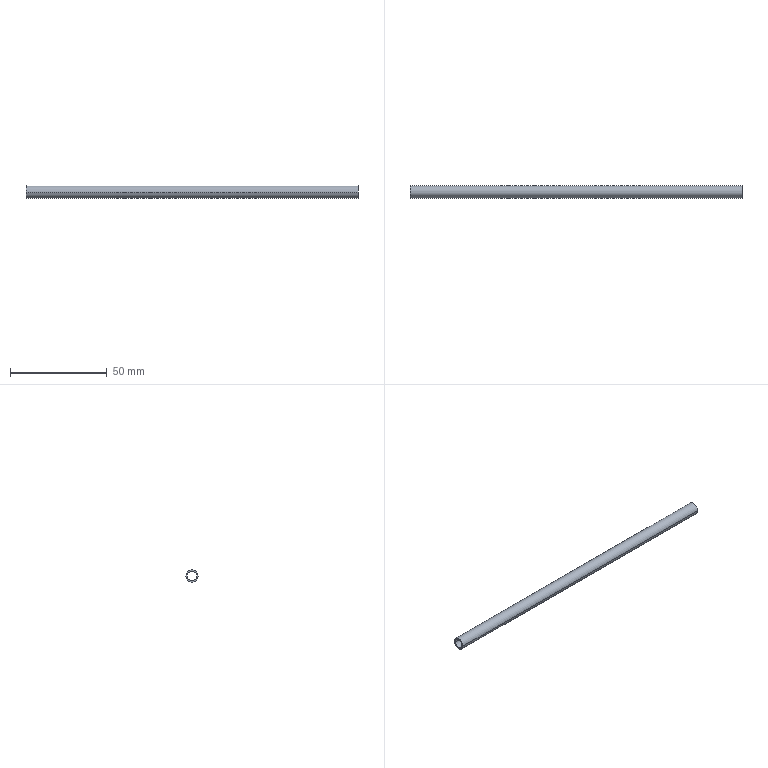Part | STEP file | copper tube 31_default_machined_ | 1 solid | 6 faces | box 172 x 6.35 x 6.35 mm | volume 2399 mm3 | cylinder 4 | plane 2 | commonest cylinder face diameters 4.75 x2 6.35 x2
STEP:
#1=CARTESIAN_POINT('',(0.,0.,0.));
#2=DIRECTION('',(0.,0.,1.));
#3=DIRECTION('',(1.,0.,0.));
#4=AXIS2_PLACEMENT_3D('',#1,#2,#3);
#5=CARTESIAN_POINT('',(-142.,3.175,0.));
#6=VERTEX_POINT('',#5);
#7=CARTESIAN_POINT('',(-142.,-3.175,0.));
#8=VERTEX_POINT('',#7);
#9=CARTESIAN_POINT('',(-142.,0.,0.));
#10=DIRECTION('',(1.,0.,0.));
#11=DIRECTION('',(0.,1.,0.));
#12=AXIS2_PLACEMENT_3D('',#9,#10,#11);
#13=CIRCLE('',#12,3.175);
#14=CARTESIAN_POINT('',(-142.,0.,0.));
#15=DIRECTION('',(1.,0.,0.));
#16=DIRECTION('',(0.,1.,0.));
#17=AXIS2_PLACEMENT_3D('',#14,#15,#16);
#18=CYLINDRICAL_SURFACE('',#17,3.175);
#19=CARTESIAN_POINT('',(0.,0.));
#20=DIRECTION('',(1.,0.));
#21=VECTOR('',#20,1.);
#22=LINE('',#19,#21);
#23=(GEOMETRIC_REPRESENTATION_CONTEXT(2)PARAMETRIC_REPRESENTATION_CONTEXT()REPRESENTATION_CONTEXT('',''));
#24=DEFINITIONAL_REPRESENTATION('',(#22),#23);
#25=PCURVE('',#18,#24);
#26=CARTESIAN_POINT('',(-142.,0.,0.));
#27=DIRECTION('',(-1.,0.,0.));
#28=DIRECTION('',(0.,-1.,0.));
#29=AXIS2_PLACEMENT_3D('',#26,#27,#28);
#30=PLANE('',#29);
#31=CARTESIAN_POINT('',(-3.175,0.));
#32=CARTESIAN_POINT('',(-3.175,5.499));
#33=CARTESIAN_POINT('',(1.587,2.75));
#34=CARTESIAN_POINT('',(6.35,0.));
#35=CARTESIAN_POINT('',(1.587,-2.75));
#36=CARTESIAN_POINT('',(-3.175,-5.499));
#37=CARTESIAN_POINT('',(-3.175,0.));
#38=(BOUNDED_CURVE()B_SPLINE_CURVE(2,(#31,#32,#33,#34,#35,#36,#37),.UNSPECIFIED.,.T.,.F.)B_SPLINE_CURVE_WITH_KNOTS((1,2,2,2,2,1),(-2.094,0.,2.094,4.189,6.283,8.378),.UNSPECIFIED.)CURVE()GEOMETRIC_REPRESENTATION_ITEM()RATIONAL_B_SPLINE_CURVE((1.,0.5,1.,0.5,1.,0.5,1.))REPRESENTATION_ITEM(''));
#39=(GEOMETRIC_REPRESENTATION_CONTEXT(2)PARAMETRIC_REPRESENTATION_CONTEXT()REPRESENTATION_CONTEXT('',''));
#40=DEFINITIONAL_REPRESENTATION('',(#38),#39);
#41=PCURVE('',#30,#40);
#42=SURFACE_CURVE('',#13,(#25,#41),.PCURVE_S1.);
#43=EDGE_CURVE('',#6,#8,#42,.T.);
#44=ORIENTED_EDGE('',*,*,#43,.T.);
#45=CARTESIAN_POINT('',(30.,-3.175,0.));
#46=VERTEX_POINT('',#45);
#47=CARTESIAN_POINT('',(-142.,-3.175,0.));
#48=DIRECTION('',(1.,0.,0.));
#49=VECTOR('',#48,1.);
#50=LINE('',#47,#49);
#51=CARTESIAN_POINT('',(3.142,0.));
#52=DIRECTION('',(0.,1.));
#53=VECTOR('',#52,1.);
#54=LINE('',#51,#53);
#55=(GEOMETRIC_REPRESENTATION_CONTEXT(2)PARAMETRIC_REPRESENTATION_CONTEXT()REPRESENTATION_CONTEXT('',''));
#56=DEFINITIONAL_REPRESENTATION('',(#54),#55);
#57=PCURVE('',#18,#56);
#58=CARTESIAN_POINT('',(-142.,0.,0.));
#59=DIRECTION('',(1.,0.,0.));
#60=DIRECTION('',(0.,1.,0.));
#61=AXIS2_PLACEMENT_3D('',#58,#59,#60);
#62=CYLINDRICAL_SURFACE('',#61,3.175);
#63=CARTESIAN_POINT('',(3.142,0.));
#64=DIRECTION('',(0.,1.));
#65=VECTOR('',#64,1.);
#66=LINE('',#63,#65);
#67=(GEOMETRIC_REPRESENTATION_CONTEXT(2)PARAMETRIC_REPRESENTATION_CONTEXT()REPRESENTATION_CONTEXT('',''));
#68=DEFINITIONAL_REPRESENTATION('',(#66),#67);
#69=PCURVE('',#62,#68);
#70=SURFACE_CURVE('',#50,(#57,#69),.PCURVE_S1.);
#71=EDGE_CURVE('',#8,#46,#70,.T.);
#72=ORIENTED_EDGE('',*,*,#71,.T.);
#73=CARTESIAN_POINT('',(30.,3.175,0.));
#74=VERTEX_POINT('',#73);
#75=CARTESIAN_POINT('',(30.,0.,0.));
#76=DIRECTION('',(1.,0.,0.));
#77=DIRECTION('',(0.,1.,0.));
#78=AXIS2_PLACEMENT_3D('',#75,#76,#77);
#79=CIRCLE('',#78,3.175);
#80=CARTESIAN_POINT('',(0.,172.));
#81=DIRECTION('',(1.,0.));
#82=VECTOR('',#81,1.);
#83=LINE('',#80,#82);
#84=(GEOMETRIC_REPRESENTATION_CONTEXT(2)PARAMETRIC_REPRESENTATION_CONTEXT()REPRESENTATION_CONTEXT('',''));
#85=DEFINITIONAL_REPRESENTATION('',(#83),#84);
#86=PCURVE('',#18,#85);
#87=CARTESIAN_POINT('',(30.,0.,0.));
#88=DIRECTION('',(1.,0.,0.));
#89=DIRECTION('',(0.,1.,0.));
#90=AXIS2_PLACEMENT_3D('',#87,#88,#89);
#91=PLANE('',#90);
#92=CARTESIAN_POINT('',(0.,0.));
#93=DIRECTION('',(1.,0.));
#94=AXIS2_PLACEMENT_2D('',#92,#93);
#95=CIRCLE('',#94,3.175);
#96=(GEOMETRIC_REPRESENTATION_CONTEXT(2)PARAMETRIC_REPRESENTATION_CONTEXT()REPRESENTATION_CONTEXT('',''));
#97=DEFINITIONAL_REPRESENTATION('',(#95),#96);
#98=PCURVE('',#91,#97);
#99=SURFACE_CURVE('',#79,(#86,#98),.PCURVE_S1.);
#100=EDGE_CURVE('',#74,#46,#99,.T.);
#101=ORIENTED_EDGE('',*,*,#100,.F.);
#102=CARTESIAN_POINT('',(-142.,3.175,0.));
#103=DIRECTION('',(1.,0.,0.));
#104=VECTOR('',#103,1.);
#105=LINE('',#102,#104);
#106=CARTESIAN_POINT('',(0.,0.));
#107=DIRECTION('',(0.,1.));
#108=VECTOR('',#107,1.);
#109=LINE('',#106,#108);
#110=(GEOMETRIC_REPRESENTATION_CONTEXT(2)PARAMETRIC_REPRESENTATION_CONTEXT()REPRESENTATION_CONTEXT('',''));
#111=DEFINITIONAL_REPRESENTATION('',(#109),#110);
#112=PCURVE('',#18,#111);
#113=CARTESIAN_POINT('',(6.283,0.));
#114=DIRECTION('',(0.,1.));
#115=VECTOR('',#114,1.);
#116=LINE('',#113,#115);
#117=(GEOMETRIC_REPRESENTATION_CONTEXT(2)PARAMETRIC_REPRESENTATION_CONTEXT()REPRESENTATION_CONTEXT('',''));
#118=DEFINITIONAL_REPRESENTATION('',(#116),#117);
#119=PCURVE('',#62,#118);
#120=SURFACE_CURVE('',#105,(#112,#119),.PCURVE_S1.);
#121=EDGE_CURVE('',#6,#74,#120,.T.);
#122=ORIENTED_EDGE('',*,*,#121,.F.);
#123=EDGE_LOOP('',(#44,#72,#101,#122));
#124=FACE_BOUND('',#123,.T.);
#125=ADVANCED_FACE('',(#124),#18,.T.);
#126=CARTESIAN_POINT('',(-142.,2.375,0.));
#127=VERTEX_POINT('',#126);
#128=CARTESIAN_POINT('',(30.,2.375,0.));
#129=VERTEX_POINT('',#128);
#130=CARTESIAN_POINT('',(-142.,2.375,0.));
#131=DIRECTION('',(1.,0.,0.));
#132=VECTOR('',#131,1.);
#133=LINE('',#130,#132);
#134=CARTESIAN_POINT('',(-142.,0.,0.));
#135=DIRECTION('',(1.,0.,0.));
#136=DIRECTION('',(0.,1.,0.));
#137=AXIS2_PLACEMENT_3D('',#134,#135,#136);
#138=CYLINDRICAL_SURFACE('',#137,2.375);
#139=CARTESIAN_POINT('',(6.283,0.));
#140=DIRECTION('',(0.,1.));
#141=VECTOR('',#140,1.);
#142=LINE('',#139,#141);
#143=(GEOMETRIC_REPRESENTATION_CONTEXT(2)PARAMETRIC_REPRESENTATION_CONTEXT()REPRESENTATION_CONTEXT('',''));
#144=DEFINITIONAL_REPRESENTATION('',(#142),#143);
#145=PCURVE('',#138,#144);
#146=CARTESIAN_POINT('',(-142.,0.,0.));
#147=DIRECTION('',(1.,0.,0.));
#148=DIRECTION('',(0.,1.,0.));
#149=AXIS2_PLACEMENT_3D('',#146,#147,#148);
#150=CYLINDRICAL_SURFACE('',#149,2.375);
#151=CARTESIAN_POINT('',(0.,0.));
#152=DIRECTION('',(0.,1.));
#153=VECTOR('',#152,1.);
#154=LINE('',#151,#153);
#155=(GEOMETRIC_REPRESENTATION_CONTEXT(2)PARAMETRIC_REPRESENTATION_CONTEXT()REPRESENTATION_CONTEXT('',''));
#156=DEFINITIONAL_REPRESENTATION('',(#154),#155);
#157=PCURVE('',#150,#156);
#158=SURFACE_CURVE('',#133,(#145,#157),.PCURVE_S1.);
#159=EDGE_CURVE('',#127,#129,#158,.T.);
#160=ORIENTED_EDGE('',*,*,#159,.T.);
#161=CARTESIAN_POINT('',(30.,-2.375,0.));
#162=VERTEX_POINT('',#161);
#163=CARTESIAN_POINT('',(30.,0.,0.));
#164=DIRECTION('',(1.,0.,0.));
#165=DIRECTION('',(0.,1.,0.));
#166=AXIS2_PLACEMENT_3D('',#163,#164,#165);
#167=CIRCLE('',#166,2.375);
#168=CARTESIAN_POINT('',(0.,172.));
#169=DIRECTION('',(1.,0.));
#170=VECTOR('',#169,1.);
#171=LINE('',#168,#170);
#172=(GEOMETRIC_REPRESENTATION_CONTEXT(2)PARAMETRIC_REPRESENTATION_CONTEXT()REPRESENTATION_CONTEXT('',''));
#173=DEFINITIONAL_REPRESENTATION('',(#171),#172);
#174=PCURVE('',#138,#173);
#175=CARTESIAN_POINT('',(0.,0.));
#176=DIRECTION('',(1.,0.));
#177=AXIS2_PLACEMENT_2D('',#175,#176);
#178=CIRCLE('',#177,2.375);
#179=(GEOMETRIC_REPRESENTATION_CONTEXT(2)PARAMETRIC_REPRESENTATION_CONTEXT()REPRESENTATION_CONTEXT('',''));
#180=DEFINITIONAL_REPRESENTATION('',(#178),#179);
#181=PCURVE('',#91,#180);
#182=SURFACE_CURVE('',#167,(#174,#181),.PCURVE_S1.);
#183=EDGE_CURVE('',#162,#129,#182,.T.);
#184=ORIENTED_EDGE('',*,*,#183,.F.);
#185=CARTESIAN_POINT('',(-142.,-2.375,0.));
#186=VERTEX_POINT('',#185);
#187=CARTESIAN_POINT('',(-142.,-2.375,0.));
#188=DIRECTION('',(1.,0.,0.));
#189=VECTOR('',#188,1.);
#190=LINE('',#187,#189);
#191=CARTESIAN_POINT('',(3.142,0.));
#192=DIRECTION('',(0.,1.));
#193=VECTOR('',#192,1.);
#194=LINE('',#191,#193);
#195=(GEOMETRIC_REPRESENTATION_CONTEXT(2)PARAMETRIC_REPRESENTATION_CONTEXT()REPRESENTATION_CONTEXT('',''));
#196=DEFINITIONAL_REPRESENTATION('',(#194),#195);
#197=PCURVE('',#138,#196);
#198=CARTESIAN_POINT('',(3.142,0.));
#199=DIRECTION('',(0.,1.));
#200=VECTOR('',#199,1.);
#201=LINE('',#198,#200);
#202=(GEOMETRIC_REPRESENTATION_CONTEXT(2)PARAMETRIC_REPRESENTATION_CONTEXT()REPRESENTATION_CONTEXT('',''));
#203=DEFINITIONAL_REPRESENTATION('',(#201),#202);
#204=PCURVE('',#150,#203);
#205=SURFACE_CURVE('',#190,(#197,#204),.PCURVE_S1.);
#206=EDGE_CURVE('',#186,#162,#205,.T.);
#207=ORIENTED_EDGE('',*,*,#206,.F.);
#208=CARTESIAN_POINT('',(-142.,0.,0.));
#209=DIRECTION('',(1.,0.,0.));
#210=DIRECTION('',(0.,1.,0.));
#211=AXIS2_PLACEMENT_3D('',#208,#209,#210);
#212=CIRCLE('',#211,2.375);
#213=CARTESIAN_POINT('',(0.,0.));
#214=DIRECTION('',(1.,0.));
#215=VECTOR('',#214,1.);
#216=LINE('',#213,#215);
#217=(GEOMETRIC_REPRESENTATION_CONTEXT(2)PARAMETRIC_REPRESENTATION_CONTEXT()REPRESENTATION_CONTEXT('',''));
#218=DEFINITIONAL_REPRESENTATION('',(#216),#217);
#219=PCURVE('',#138,#218);
#220=CARTESIAN_POINT('',(-2.375,0.));
#221=CARTESIAN_POINT('',(-2.375,4.114));
#222=CARTESIAN_POINT('',(1.188,2.057));
#223=CARTESIAN_POINT('',(4.75,0.));
#224=CARTESIAN_POINT('',(1.188,-2.057));
#225=CARTESIAN_POINT('',(-2.375,-4.114));
#226=CARTESIAN_POINT('',(-2.375,0.));
#227=(BOUNDED_CURVE()B_SPLINE_CURVE(2,(#220,#221,#222,#223,#224,#225,#226),.UNSPECIFIED.,.T.,.F.)B_SPLINE_CURVE_WITH_KNOTS((1,2,2,2,2,1),(-2.094,0.,2.094,4.189,6.283,8.378),.UNSPECIFIED.)CURVE()GEOMETRIC_REPRESENTATION_ITEM()RATIONAL_B_SPLINE_CURVE((1.,0.5,1.,0.5,1.,0.5,1.))REPRESENTATION_ITEM(''));
#228=(GEOMETRIC_REPRESENTATION_CONTEXT(2)PARAMETRIC_REPRESENTATION_CONTEXT()REPRESENTATION_CONTEXT('',''));
#229=DEFINITIONAL_REPRESENTATION('',(#227),#228);
#230=PCURVE('',#30,#229);
#231=SURFACE_CURVE('',#212,(#219,#230),.PCURVE_S1.);
#232=EDGE_CURVE('',#186,#127,#231,.T.);
#233=ORIENTED_EDGE('',*,*,#232,.T.);
#234=EDGE_LOOP('',(#160,#184,#207,#233));
#235=FACE_BOUND('',#234,.F.);
#236=ADVANCED_FACE('',(#235),#138,.F.);
#237=ORIENTED_EDGE('',*,*,#71,.F.);
#238=CARTESIAN_POINT('',(-142.,0.,0.));
#239=DIRECTION('',(1.,0.,0.));
#240=DIRECTION('',(0.,1.,0.));
#241=AXIS2_PLACEMENT_3D('',#238,#239,#240);
#242=CIRCLE('',#241,3.175);
#243=CARTESIAN_POINT('',(0.,0.));
#244=DIRECTION('',(1.,0.));
#245=VECTOR('',#244,1.);
#246=LINE('',#243,#245);
#247=(GEOMETRIC_REPRESENTATION_CONTEXT(2)PARAMETRIC_REPRESENTATION_CONTEXT()REPRESENTATION_CONTEXT('',''));
#248=DEFINITIONAL_REPRESENTATION('',(#246),#247);
#249=PCURVE('',#62,#248);
#250=CARTESIAN_POINT('',(-3.175,0.));
#251=CARTESIAN_POINT('',(-3.175,5.499));
#252=CARTESIAN_POINT('',(1.587,2.75));
#253=CARTESIAN_POINT('',(6.35,0.));
#254=CARTESIAN_POINT('',(1.587,-2.75));
#255=CARTESIAN_POINT('',(-3.175,-5.499));
#256=CARTESIAN_POINT('',(-3.175,0.));
#257=(BOUNDED_CURVE()B_SPLINE_CURVE(2,(#250,#251,#252,#253,#254,#255,#256),.UNSPECIFIED.,.T.,.F.)B_SPLINE_CURVE_WITH_KNOTS((1,2,2,2,2,1),(-2.094,0.,2.094,4.189,6.283,8.378),.UNSPECIFIED.)CURVE()GEOMETRIC_REPRESENTATION_ITEM()RATIONAL_B_SPLINE_CURVE((1.,0.5,1.,0.5,1.,0.5,1.))REPRESENTATION_ITEM(''));
#258=(GEOMETRIC_REPRESENTATION_CONTEXT(2)PARAMETRIC_REPRESENTATION_CONTEXT()REPRESENTATION_CONTEXT('',''));
#259=DEFINITIONAL_REPRESENTATION('',(#257),#258);
#260=PCURVE('',#30,#259);
#261=SURFACE_CURVE('',#242,(#249,#260),.PCURVE_S1.);
#262=EDGE_CURVE('',#8,#6,#261,.T.);
#263=ORIENTED_EDGE('',*,*,#262,.T.);
#264=ORIENTED_EDGE('',*,*,#121,.T.);
#265=CARTESIAN_POINT('',(30.,0.,0.));
#266=DIRECTION('',(1.,0.,0.));
#267=DIRECTION('',(0.,1.,0.));
#268=AXIS2_PLACEMENT_3D('',#265,#266,#267);
#269=CIRCLE('',#268,3.175);
#270=CARTESIAN_POINT('',(0.,172.));
#271=DIRECTION('',(1.,0.));
#272=VECTOR('',#271,1.);
#273=LINE('',#270,#272);
#274=(GEOMETRIC_REPRESENTATION_CONTEXT(2)PARAMETRIC_REPRESENTATION_CONTEXT()REPRESENTATION_CONTEXT('',''));
#275=DEFINITIONAL_REPRESENTATION('',(#273),#274);
#276=PCURVE('',#62,#275);
#277=CARTESIAN_POINT('',(0.,0.));
#278=DIRECTION('',(1.,0.));
#279=AXIS2_PLACEMENT_2D('',#277,#278);
#280=CIRCLE('',#279,3.175);
#281=(GEOMETRIC_REPRESENTATION_CONTEXT(2)PARAMETRIC_REPRESENTATION_CONTEXT()REPRESENTATION_CONTEXT('',''));
#282=DEFINITIONAL_REPRESENTATION('',(#280),#281);
#283=PCURVE('',#91,#282);
#284=SURFACE_CURVE('',#269,(#276,#283),.PCURVE_S1.);
#285=EDGE_CURVE('',#46,#74,#284,.T.);
#286=ORIENTED_EDGE('',*,*,#285,.F.);
#287=EDGE_LOOP('',(#237,#263,#264,#286));
#288=FACE_BOUND('',#287,.T.);
#289=ADVANCED_FACE('',(#288),#62,.T.);
#290=ORIENTED_EDGE('',*,*,#43,.F.);
#291=ORIENTED_EDGE('',*,*,#262,.F.);
#292=EDGE_LOOP('',(#290,#291));
#293=FACE_BOUND('',#292,.T.);
#294=CARTESIAN_POINT('',(-142.,0.,0.));
#295=DIRECTION('',(1.,0.,0.));
#296=DIRECTION('',(0.,1.,0.));
#297=AXIS2_PLACEMENT_3D('',#294,#295,#296);
#298=CIRCLE('',#297,2.375);
#299=CARTESIAN_POINT('',(-2.375,0.));
#300=CARTESIAN_POINT('',(-2.375,4.114));
#301=CARTESIAN_POINT('',(1.188,2.057));
#302=CARTESIAN_POINT('',(4.75,0.));
#303=CARTESIAN_POINT('',(1.188,-2.057));
#304=CARTESIAN_POINT('',(-2.375,-4.114));
#305=CARTESIAN_POINT('',(-2.375,0.));
#306=(BOUNDED_CURVE()B_SPLINE_CURVE(2,(#299,#300,#301,#302,#303,#304,#305),.UNSPECIFIED.,.T.,.F.)B_SPLINE_CURVE_WITH_KNOTS((1,2,2,2,2,1),(-2.094,0.,2.094,4.189,6.283,8.378),.UNSPECIFIED.)CURVE()GEOMETRIC_REPRESENTATION_ITEM()RATIONAL_B_SPLINE_CURVE((1.,0.5,1.,0.5,1.,0.5,1.))REPRESENTATION_ITEM(''));
#307=(GEOMETRIC_REPRESENTATION_CONTEXT(2)PARAMETRIC_REPRESENTATION_CONTEXT()REPRESENTATION_CONTEXT('',''));
#308=DEFINITIONAL_REPRESENTATION('',(#306),#307);
#309=PCURVE('',#30,#308);
#310=CARTESIAN_POINT('',(0.,0.));
#311=DIRECTION('',(1.,0.));
#312=VECTOR('',#311,1.);
#313=LINE('',#310,#312);
#314=(GEOMETRIC_REPRESENTATION_CONTEXT(2)PARAMETRIC_REPRESENTATION_CONTEXT()REPRESENTATION_CONTEXT('',''));
#315=DEFINITIONAL_REPRESENTATION('',(#313),#314);
#316=PCURVE('',#150,#315);
#317=SURFACE_CURVE('',#298,(#309,#316),.PCURVE_S1.);
#318=EDGE_CURVE('',#127,#186,#317,.T.);
#319=ORIENTED_EDGE('',*,*,#318,.T.);
#320=ORIENTED_EDGE('',*,*,#232,.T.);
#321=EDGE_LOOP('',(#319,#320));
#322=FACE_BOUND('',#321,.T.);
#323=ADVANCED_FACE('',(#293,#322),#30,.T.);
#324=CARTESIAN_POINT('',(30.,0.,0.));
#325=DIRECTION('',(1.,0.,0.));
#326=DIRECTION('',(0.,1.,0.));
#327=AXIS2_PLACEMENT_3D('',#324,#325,#326);
#328=CIRCLE('',#327,2.375);
#329=CARTESIAN_POINT('',(0.,172.));
#330=DIRECTION('',(1.,0.));
#331=VECTOR('',#330,1.);
#332=LINE('',#329,#331);
#333=(GEOMETRIC_REPRESENTATION_CONTEXT(2)PARAMETRIC_REPRESENTATION_CONTEXT()REPRESENTATION_CONTEXT('',''));
#334=DEFINITIONAL_REPRESENTATION('',(#332),#333);
#335=PCURVE('',#150,#334);
#336=CARTESIAN_POINT('',(0.,0.));
#337=DIRECTION('',(1.,0.));
#338=AXIS2_PLACEMENT_2D('',#336,#337);
#339=CIRCLE('',#338,2.375);
#340=(GEOMETRIC_REPRESENTATION_CONTEXT(2)PARAMETRIC_REPRESENTATION_CONTEXT()REPRESENTATION_CONTEXT('',''));
#341=DEFINITIONAL_REPRESENTATION('',(#339),#340);
#342=PCURVE('',#91,#341);
#343=SURFACE_CURVE('',#328,(#335,#342),.PCURVE_S1.);
#344=EDGE_CURVE('',#129,#162,#343,.T.);
#345=ORIENTED_EDGE('',*,*,#344,.F.);
#346=ORIENTED_EDGE('',*,*,#159,.F.);
#347=ORIENTED_EDGE('',*,*,#318,.T.);
#348=ORIENTED_EDGE('',*,*,#206,.T.);
#349=EDGE_LOOP('',(#345,#346,#347,#348));
#350=FACE_BOUND('',#349,.F.);
#351=ADVANCED_FACE('',(#350),#150,.F.);
#352=ORIENTED_EDGE('',*,*,#100,.T.);
#353=ORIENTED_EDGE('',*,*,#285,.T.);
#354=EDGE_LOOP('',(#352,#353));
#355=FACE_BOUND('',#354,.T.);
#356=ORIENTED_EDGE('',*,*,#344,.F.);
#357=ORIENTED_EDGE('',*,*,#183,.F.);
#358=EDGE_LOOP('',(#356,#357));
#359=FACE_BOUND('',#358,.T.);
#360=ADVANCED_FACE('',(#355,#359),#91,.T.);
#361=CLOSED_SHELL('',(#125,#236,#289,#323,#351,#360));
#362=MANIFOLD_SOLID_BREP('',#361);
#363=(LENGTH_UNIT()NAMED_UNIT(*)SI_UNIT(.MILLI.,.METRE.));
#364=UNCERTAINTY_MEASURE_WITH_UNIT(LENGTH_MEASURE(0.0000001),#363,'','');
#365=(NAMED_UNIT(*)PLANE_ANGLE_UNIT()SI_UNIT($,.RADIAN.));
#366=(NAMED_UNIT(*)SI_UNIT($,.STERADIAN.)SOLID_ANGLE_UNIT());
#367=(GEOMETRIC_REPRESENTATION_CONTEXT(3)GLOBAL_UNCERTAINTY_ASSIGNED_CONTEXT((#364))GLOBAL_UNIT_ASSIGNED_CONTEXT((#363,#365,#366))REPRESENTATION_CONTEXT('',''));
#368=ADVANCED_BREP_SHAPE_REPRESENTATION('',(#4,#362),#367);